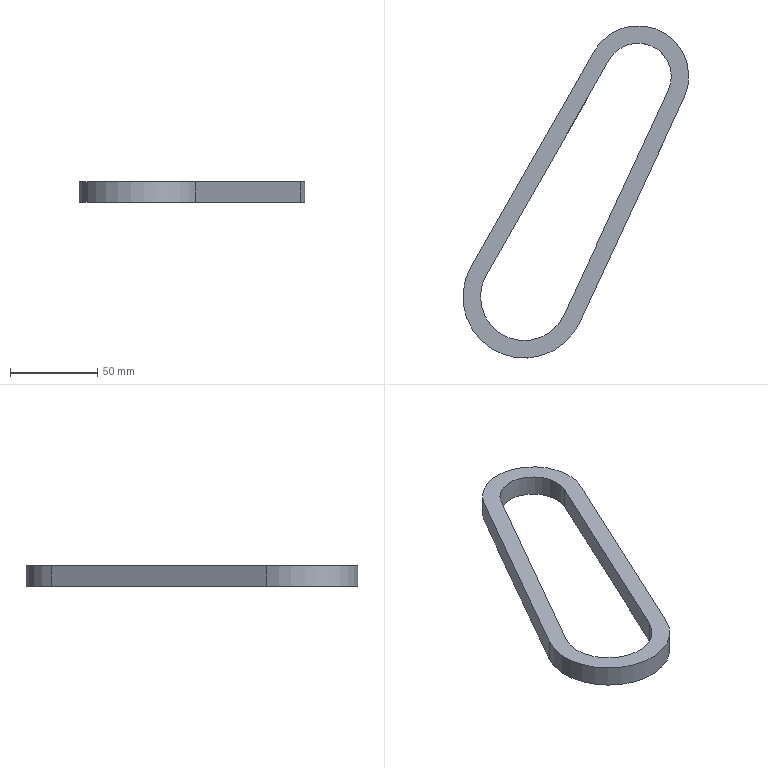Part | NX | 1 solid | 10 faces | box 129.118 x 190 x 12 mm | volume 54428 mm3 | plane 6 | cylinder 4 | commonest cylinder face diameters 38 x1 50 x1 58 x1 70 x1
STEP:
#1=CARTESIAN_POINT('',(1422.233,-8.001,161.));
#2=VERTEX_POINT('',#1);
#3=CARTESIAN_POINT('',(1388.505,9.43,161.));
#4=VERTEX_POINT('',#3);
#5=CARTESIAN_POINT('',(1405.,0.,161.));
#6=DIRECTION('',(0.,0.,1.));
#7=DIRECTION('',(0.907,-0.4211,0.));
#8=AXIS2_PLACEMENT_3D('',#5,#6,#7);
#9=CIRCLE('',#8,19.);
#10=EDGE_CURVE('',#2,#4,#9,.T.);
#11=ORIENTED_EDGE('',*,*,#10,.T.);
#12=CARTESIAN_POINT('',(1388.505,9.43,149.));
#13=VERTEX_POINT('',#12);
#14=CARTESIAN_POINT('',(1388.505,9.43,161.));
#15=DIRECTION('',(0.,0.,-1.));
#16=VECTOR('',#15,1.);
#17=LINE('',#14,#16);
#18=EDGE_CURVE('',#4,#13,#17,.T.);
#19=ORIENTED_EDGE('',*,*,#18,.T.);
#20=CARTESIAN_POINT('',(1422.233,-8.001,149.));
#21=VERTEX_POINT('',#20);
#22=CARTESIAN_POINT('',(1405.,0.,149.));
#23=DIRECTION('',(0.,0.,1.));
#24=DIRECTION('',(0.907,-0.4211,0.));
#25=AXIS2_PLACEMENT_3D('',#22,#23,#24);
#26=CIRCLE('',#25,19.);
#27=EDGE_CURVE('',#21,#13,#26,.T.);
#28=ORIENTED_EDGE('',*,*,#27,.F.);
#29=CARTESIAN_POINT('',(1422.233,-8.001,161.));
#30=DIRECTION('',(0.,0.,-1.));
#31=VECTOR('',#30,1.);
#32=LINE('',#29,#31);
#33=EDGE_CURVE('',#2,#21,#32,.T.);
#34=ORIENTED_EDGE('',*,*,#33,.F.);
#35=EDGE_LOOP('',(#11,#19,#28,#34));
#36=FACE_OUTER_BOUND('',#35,.T.);
#37=CARTESIAN_POINT('',(1405.,0.,161.));
#38=DIRECTION('',(0.,0.,1.));
#39=DIRECTION('',(1.,0.,0.));
#40=AXIS2_PLACEMENT_3D('',#37,#38,#39);
#41=CYLINDRICAL_SURFACE('',#40,19.);
#42=ADVANCED_FACE('',(#36),#41,.F.);
#43=CARTESIAN_POINT('',(1362.557,-136.528,161.));
#44=VERTEX_POINT('',#43);
#45=CARTESIAN_POINT('',(1362.557,-136.528,161.));
#46=DIRECTION('',(0.4211,0.907,0.));
#47=VECTOR('',#46,1.);
#48=LINE('',#45,#47);
#49=EDGE_CURVE('',#44,#2,#48,.T.);
#50=ORIENTED_EDGE('',*,*,#49,.T.);
#51=ORIENTED_EDGE('',*,*,#33,.T.);
#52=CARTESIAN_POINT('',(1362.557,-136.528,149.));
#53=VERTEX_POINT('',#52);
#54=CARTESIAN_POINT('',(1362.557,-136.528,149.));
#55=DIRECTION('',(0.4211,0.907,0.));
#56=VECTOR('',#55,1.);
#57=LINE('',#54,#56);
#58=EDGE_CURVE('',#53,#21,#57,.T.);
#59=ORIENTED_EDGE('',*,*,#58,.F.);
#60=CARTESIAN_POINT('',(1362.557,-136.528,161.));
#61=DIRECTION('',(0.,0.,-1.));
#62=VECTOR('',#61,1.);
#63=LINE('',#60,#62);
#64=EDGE_CURVE('',#44,#53,#63,.T.);
#65=ORIENTED_EDGE('',*,*,#64,.F.);
#66=EDGE_LOOP('',(#50,#51,#59,#65));
#67=FACE_OUTER_BOUND('',#66,.T.);
#68=CARTESIAN_POINT('',(1362.557,-136.528,161.));
#69=DIRECTION('',(0.907,-0.4211,0.));
#70=DIRECTION('',(0.,0.,-1.));
#71=AXIS2_PLACEMENT_3D('',#68,#69,#70);
#72=PLANE('',#71);
#73=ADVANCED_FACE('',(#67),#72,.F.);
#74=CARTESIAN_POINT('',(1318.178,-113.593,161.));
#75=VERTEX_POINT('',#74);
#76=CARTESIAN_POINT('',(1339.882,-126.,161.));
#77=DIRECTION('',(0.,0.,1.));
#78=DIRECTION('',(-0.8682,0.4963,0.));
#79=AXIS2_PLACEMENT_3D('',#76,#77,#78);
#80=CIRCLE('',#79,25.);
#81=EDGE_CURVE('',#75,#44,#80,.T.);
#82=ORIENTED_EDGE('',*,*,#81,.T.);
#83=ORIENTED_EDGE('',*,*,#64,.T.);
#84=CARTESIAN_POINT('',(1318.178,-113.593,149.));
#85=VERTEX_POINT('',#84);
#86=CARTESIAN_POINT('',(1339.882,-126.,149.));
#87=DIRECTION('',(0.,0.,1.));
#88=DIRECTION('',(-0.8682,0.4963,0.));
#89=AXIS2_PLACEMENT_3D('',#86,#87,#88);
#90=CIRCLE('',#89,25.);
#91=EDGE_CURVE('',#85,#53,#90,.T.);
#92=ORIENTED_EDGE('',*,*,#91,.F.);
#93=CARTESIAN_POINT('',(1318.178,-113.593,161.));
#94=DIRECTION('',(0.,0.,-1.));
#95=VECTOR('',#94,1.);
#96=LINE('',#93,#95);
#97=EDGE_CURVE('',#75,#85,#96,.T.);
#98=ORIENTED_EDGE('',*,*,#97,.F.);
#99=EDGE_LOOP('',(#82,#83,#92,#98));
#100=FACE_OUTER_BOUND('',#99,.T.);
#101=CARTESIAN_POINT('',(1339.882,-126.,161.));
#102=DIRECTION('',(0.,0.,1.));
#103=DIRECTION('',(1.,0.,0.));
#104=AXIS2_PLACEMENT_3D('',#101,#102,#103);
#105=CYLINDRICAL_SURFACE('',#104,25.);
#106=ADVANCED_FACE('',(#100),#105,.F.);
#107=CARTESIAN_POINT('',(1388.505,9.43,161.));
#108=DIRECTION('',(-0.4963,-0.8682,0.));
#109=VECTOR('',#108,1.);
#110=LINE('',#107,#109);
#111=EDGE_CURVE('',#4,#75,#110,.T.);
#112=ORIENTED_EDGE('',*,*,#111,.T.);
#113=ORIENTED_EDGE('',*,*,#97,.T.);
#114=CARTESIAN_POINT('',(1388.505,9.43,149.));
#115=DIRECTION('',(-0.4963,-0.8682,0.));
#116=VECTOR('',#115,1.);
#117=LINE('',#114,#116);
#118=EDGE_CURVE('',#13,#85,#117,.T.);
#119=ORIENTED_EDGE('',*,*,#118,.F.);
#120=ORIENTED_EDGE('',*,*,#18,.F.);
#121=EDGE_LOOP('',(#112,#113,#119,#120));
#122=FACE_OUTER_BOUND('',#121,.T.);
#123=CARTESIAN_POINT('',(1388.505,9.43,161.));
#124=DIRECTION('',(-0.8682,0.4963,0.));
#125=DIRECTION('',(0.,0.,1.));
#126=AXIS2_PLACEMENT_3D('',#123,#124,#125);
#127=PLANE('',#126);
#128=ADVANCED_FACE('',(#122),#127,.F.);
#129=CARTESIAN_POINT('',(1379.823,14.392,161.));
#130=VERTEX_POINT('',#129);
#131=CARTESIAN_POINT('',(1309.497,-108.63,161.));
#132=VERTEX_POINT('',#131);
#133=CARTESIAN_POINT('',(1379.823,14.392,161.));
#134=DIRECTION('',(-0.4963,-0.8682,0.));
#135=VECTOR('',#134,1.);
#136=LINE('',#133,#135);
#137=EDGE_CURVE('',#130,#132,#136,.T.);
#138=ORIENTED_EDGE('',*,*,#137,.T.);
#139=CARTESIAN_POINT('',(1371.627,-140.739,161.));
#140=VERTEX_POINT('',#139);
#141=CARTESIAN_POINT('',(1339.882,-126.,161.));
#142=DIRECTION('',(0.,0.,1.));
#143=DIRECTION('',(-0.8682,0.4963,0.));
#144=AXIS2_PLACEMENT_3D('',#141,#142,#143);
#145=CIRCLE('',#144,35.);
#146=EDGE_CURVE('',#132,#140,#145,.T.);
#147=ORIENTED_EDGE('',*,*,#146,.T.);
#148=CARTESIAN_POINT('',(1431.303,-12.213,161.));
#149=VERTEX_POINT('',#148);
#150=CARTESIAN_POINT('',(1371.627,-140.739,161.));
#151=DIRECTION('',(0.4211,0.907,0.));
#152=VECTOR('',#151,1.);
#153=LINE('',#150,#152);
#154=EDGE_CURVE('',#140,#149,#153,.T.);
#155=ORIENTED_EDGE('',*,*,#154,.T.);
#156=CARTESIAN_POINT('',(1405.,0.,161.));
#157=DIRECTION('',(0.,0.,1.));
#158=DIRECTION('',(0.907,-0.4211,0.));
#159=AXIS2_PLACEMENT_3D('',#156,#157,#158);
#160=CIRCLE('',#159,29.);
#161=EDGE_CURVE('',#149,#130,#160,.T.);
#162=ORIENTED_EDGE('',*,*,#161,.T.);
#163=EDGE_LOOP('',(#138,#147,#155,#162));
#164=FACE_BOUND('',#163,.T.);
#165=ORIENTED_EDGE('',*,*,#49,.F.);
#166=ORIENTED_EDGE('',*,*,#81,.F.);
#167=ORIENTED_EDGE('',*,*,#111,.F.);
#168=ORIENTED_EDGE('',*,*,#10,.F.);
#169=EDGE_LOOP('',(#165,#166,#167,#168));
#170=FACE_BOUND('',#169,.T.);
#171=CARTESIAN_POINT('',(1416.019,21.321,161.));
#172=DIRECTION('',(0.,0.,1.));
#173=DIRECTION('',(1.,0.,0.));
#174=AXIS2_PLACEMENT_3D('',#171,#172,#173);
#175=PLANE('',#174);
#176=ADVANCED_FACE('',(#164,#170),#175,.T.);
#177=CARTESIAN_POINT('',(1371.627,-140.739,149.));
#178=VERTEX_POINT('',#177);
#179=CARTESIAN_POINT('',(1431.303,-12.213,149.));
#180=VERTEX_POINT('',#179);
#181=CARTESIAN_POINT('',(1371.627,-140.739,149.));
#182=DIRECTION('',(0.4211,0.907,0.));
#183=VECTOR('',#182,1.);
#184=LINE('',#181,#183);
#185=EDGE_CURVE('',#178,#180,#184,.T.);
#186=ORIENTED_EDGE('',*,*,#185,.F.);
#187=CARTESIAN_POINT('',(1309.497,-108.63,149.));
#188=VERTEX_POINT('',#187);
#189=CARTESIAN_POINT('',(1339.882,-126.,149.));
#190=DIRECTION('',(0.,0.,1.));
#191=DIRECTION('',(-0.8682,0.4963,0.));
#192=AXIS2_PLACEMENT_3D('',#189,#190,#191);
#193=CIRCLE('',#192,35.);
#194=EDGE_CURVE('',#188,#178,#193,.T.);
#195=ORIENTED_EDGE('',*,*,#194,.F.);
#196=CARTESIAN_POINT('',(1379.823,14.392,149.));
#197=VERTEX_POINT('',#196);
#198=CARTESIAN_POINT('',(1379.823,14.392,149.));
#199=DIRECTION('',(-0.4963,-0.8682,0.));
#200=VECTOR('',#199,1.);
#201=LINE('',#198,#200);
#202=EDGE_CURVE('',#197,#188,#201,.T.);
#203=ORIENTED_EDGE('',*,*,#202,.F.);
#204=CARTESIAN_POINT('',(1405.,0.,149.));
#205=DIRECTION('',(0.,0.,1.));
#206=DIRECTION('',(0.907,-0.4211,0.));
#207=AXIS2_PLACEMENT_3D('',#204,#205,#206);
#208=CIRCLE('',#207,29.);
#209=EDGE_CURVE('',#180,#197,#208,.T.);
#210=ORIENTED_EDGE('',*,*,#209,.F.);
#211=EDGE_LOOP('',(#186,#195,#203,#210));
#212=FACE_BOUND('',#211,.T.);
#213=ORIENTED_EDGE('',*,*,#118,.T.);
#214=ORIENTED_EDGE('',*,*,#91,.T.);
#215=ORIENTED_EDGE('',*,*,#58,.T.);
#216=ORIENTED_EDGE('',*,*,#27,.T.);
#217=EDGE_LOOP('',(#213,#214,#215,#216));
#218=FACE_BOUND('',#217,.T.);
#219=CARTESIAN_POINT('',(1416.019,21.321,149.));
#220=DIRECTION('',(0.,0.,1.));
#221=DIRECTION('',(1.,0.,0.));
#222=AXIS2_PLACEMENT_3D('',#219,#220,#221);
#223=PLANE('',#222);
#224=ADVANCED_FACE('',(#212,#218),#223,.F.);
#225=ORIENTED_EDGE('',*,*,#161,.F.);
#226=CARTESIAN_POINT('',(1431.303,-12.213,161.));
#227=DIRECTION('',(0.,0.,-1.));
#228=VECTOR('',#227,1.);
#229=LINE('',#226,#228);
#230=EDGE_CURVE('',#149,#180,#229,.T.);
#231=ORIENTED_EDGE('',*,*,#230,.T.);
#232=ORIENTED_EDGE('',*,*,#209,.T.);
#233=CARTESIAN_POINT('',(1379.823,14.392,161.));
#234=DIRECTION('',(0.,0.,-1.));
#235=VECTOR('',#234,1.);
#236=LINE('',#233,#235);
#237=EDGE_CURVE('',#130,#197,#236,.T.);
#238=ORIENTED_EDGE('',*,*,#237,.F.);
#239=EDGE_LOOP('',(#225,#231,#232,#238));
#240=FACE_OUTER_BOUND('',#239,.T.);
#241=CARTESIAN_POINT('',(1405.,0.,161.));
#242=DIRECTION('',(0.,0.,1.));
#243=DIRECTION('',(1.,0.,0.));
#244=AXIS2_PLACEMENT_3D('',#241,#242,#243);
#245=CYLINDRICAL_SURFACE('',#244,29.);
#246=ADVANCED_FACE('',(#240),#245,.T.);
#247=ORIENTED_EDGE('',*,*,#154,.F.);
#248=CARTESIAN_POINT('',(1371.627,-140.739,161.));
#249=DIRECTION('',(0.,0.,-1.));
#250=VECTOR('',#249,1.);
#251=LINE('',#248,#250);
#252=EDGE_CURVE('',#140,#178,#251,.T.);
#253=ORIENTED_EDGE('',*,*,#252,.T.);
#254=ORIENTED_EDGE('',*,*,#185,.T.);
#255=ORIENTED_EDGE('',*,*,#230,.F.);
#256=EDGE_LOOP('',(#247,#253,#254,#255));
#257=FACE_OUTER_BOUND('',#256,.T.);
#258=CARTESIAN_POINT('',(1371.627,-140.739,161.));
#259=DIRECTION('',(0.907,-0.4211,0.));
#260=DIRECTION('',(0.,0.,-1.));
#261=AXIS2_PLACEMENT_3D('',#258,#259,#260);
#262=PLANE('',#261);
#263=ADVANCED_FACE('',(#257),#262,.T.);
#264=ORIENTED_EDGE('',*,*,#146,.F.);
#265=CARTESIAN_POINT('',(1309.497,-108.63,161.));
#266=DIRECTION('',(0.,0.,-1.));
#267=VECTOR('',#266,1.);
#268=LINE('',#265,#267);
#269=EDGE_CURVE('',#132,#188,#268,.T.);
#270=ORIENTED_EDGE('',*,*,#269,.T.);
#271=ORIENTED_EDGE('',*,*,#194,.T.);
#272=ORIENTED_EDGE('',*,*,#252,.F.);
#273=EDGE_LOOP('',(#264,#270,#271,#272));
#274=FACE_OUTER_BOUND('',#273,.T.);
#275=CARTESIAN_POINT('',(1339.882,-126.,161.));
#276=DIRECTION('',(0.,0.,1.));
#277=DIRECTION('',(1.,0.,0.));
#278=AXIS2_PLACEMENT_3D('',#275,#276,#277);
#279=CYLINDRICAL_SURFACE('',#278,35.);
#280=ADVANCED_FACE('',(#274),#279,.T.);
#281=ORIENTED_EDGE('',*,*,#137,.F.);
#282=ORIENTED_EDGE('',*,*,#237,.T.);
#283=ORIENTED_EDGE('',*,*,#202,.T.);
#284=ORIENTED_EDGE('',*,*,#269,.F.);
#285=EDGE_LOOP('',(#281,#282,#283,#284));
#286=FACE_OUTER_BOUND('',#285,.T.);
#287=CARTESIAN_POINT('',(1379.823,14.392,161.));
#288=DIRECTION('',(-0.8682,0.4963,0.));
#289=DIRECTION('',(0.,0.,1.));
#290=AXIS2_PLACEMENT_3D('',#287,#288,#289);
#291=PLANE('',#290);
#292=ADVANCED_FACE('',(#286),#291,.T.);
#293=CLOSED_SHELL('',(#42,#73,#106,#128,#176,#224,#246,#263,#280,#292));
#294=MANIFOLD_SOLID_BREP('',#293);
#295=(LENGTH_UNIT()NAMED_UNIT(*)SI_UNIT(.MILLI.,.METRE.));
#296=UNCERTAINTY_MEASURE_WITH_UNIT(LENGTH_MEASURE(0.00002),#295,'','');
#297=(NAMED_UNIT(*)PLANE_ANGLE_UNIT()SI_UNIT($,.RADIAN.));
#298=PLANE_ANGLE_MEASURE_WITH_UNIT(PLANE_ANGLE_MEASURE(0.01745),#297);
#299=DIMENSIONAL_EXPONENTS(0.,0.,0.,0.,0.,0.,0.);
#300=(CONVERSION_BASED_UNIT('DEGREE',#298)NAMED_UNIT(#299)PLANE_ANGLE_UNIT());
#301=(NAMED_UNIT(*)SI_UNIT($,.STERADIAN.)SOLID_ANGLE_UNIT());
#302=(GEOMETRIC_REPRESENTATION_CONTEXT(3)GLOBAL_UNCERTAINTY_ASSIGNED_CONTEXT((#296))GLOBAL_UNIT_ASSIGNED_CONTEXT((#295,#300,#301))REPRESENTATION_CONTEXT('',''));
#303=ADVANCED_BREP_SHAPE_REPRESENTATION('',(#294),#302);